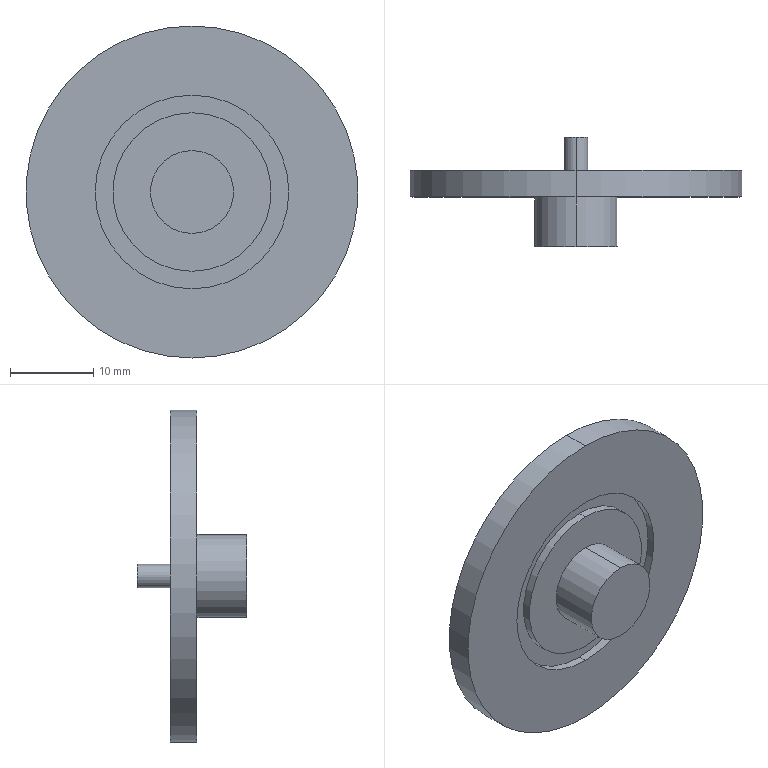Part | SolidWorks | features ICE 5, Extrusion 1 | 1 solid | 28 faces | box 40 x 13.2 x 40 mm | volume 4095 mm3 | cylinder 18 | plane 10 | commonest cylinder face diameters 2.85 x2 10 x2 16.818 x2 19.091 x2 20.068 x2 23.339 x2
STEP:
#1=CARTESIAN_POINT('',(0.,7.2,1.425));
#2=VERTEX_POINT('',#1);
#3=CARTESIAN_POINT('',(0.,7.2,-1.425));
#4=VERTEX_POINT('',#3);
#5=CARTESIAN_POINT('',(0.,7.2,0.));
#6=DIRECTION('',(0.,1.,0.));
#7=DIRECTION('',(0.,0.,1.));
#8=AXIS2_PLACEMENT_3D('',#5,#6,#7);
#9=CIRCLE('',#8,1.425);
#10=EDGE_CURVE('',#2,#4,#9,.T.);
#11=ORIENTED_EDGE('',*,*,#10,.F.);
#12=CARTESIAN_POINT('',(0.,3.2,1.425));
#13=VERTEX_POINT('',#12);
#14=CARTESIAN_POINT('',(0.,7.2,1.425));
#15=DIRECTION('',(0.,-1.,0.));
#16=VECTOR('',#15,1000.);
#17=LINE('',#14,#16);
#18=EDGE_CURVE('',#2,#13,#17,.T.);
#19=ORIENTED_EDGE('',*,*,#18,.T.);
#20=CARTESIAN_POINT('',(0.,3.2,-1.425));
#21=VERTEX_POINT('',#20);
#22=CARTESIAN_POINT('',(0.,3.2,0.));
#23=DIRECTION('',(0.,1.,0.));
#24=DIRECTION('',(0.,0.,1.));
#25=AXIS2_PLACEMENT_3D('',#22,#23,#24);
#26=CIRCLE('',#25,1.425);
#27=EDGE_CURVE('',#13,#21,#26,.T.);
#28=ORIENTED_EDGE('',*,*,#27,.T.);
#29=CARTESIAN_POINT('',(0.,7.2,-1.425));
#30=DIRECTION('',(0.,-1.,0.));
#31=VECTOR('',#30,1000.);
#32=LINE('',#29,#31);
#33=EDGE_CURVE('',#4,#21,#32,.T.);
#34=ORIENTED_EDGE('',*,*,#33,.F.);
#35=EDGE_LOOP('',(#11,#19,#28,#34));
#36=FACE_OUTER_BOUND('',#35,.T.);
#37=CARTESIAN_POINT('',(0.,7.2,0.));
#38=DIRECTION('',(0.,-1.,0.));
#39=DIRECTION('',(0.,0.,-1.));
#40=AXIS2_PLACEMENT_3D('',#37,#38,#39);
#41=CYLINDRICAL_SURFACE('',#40,1.425);
#42=ADVANCED_FACE('',(#36),#41,.T.);
#43=CARTESIAN_POINT('',(0.,2.2,8.409));
#44=VERTEX_POINT('',#43);
#45=CARTESIAN_POINT('',(0.,2.2,-8.409));
#46=VERTEX_POINT('',#45);
#47=CARTESIAN_POINT('',(0.,2.2,0.));
#48=DIRECTION('',(0.,1.,0.));
#49=DIRECTION('',(0.,0.,1.));
#50=AXIS2_PLACEMENT_3D('',#47,#48,#49);
#51=CIRCLE('',#50,8.409);
#52=EDGE_CURVE('',#44,#46,#51,.T.);
#53=ORIENTED_EDGE('',*,*,#52,.T.);
#54=CARTESIAN_POINT('',(0.,3.2,-8.409));
#55=VERTEX_POINT('',#54);
#56=CARTESIAN_POINT('',(0.,2.2,-8.409));
#57=DIRECTION('',(0.,1.,0.));
#58=VECTOR('',#57,1000.);
#59=LINE('',#56,#58);
#60=EDGE_CURVE('',#46,#55,#59,.T.);
#61=ORIENTED_EDGE('',*,*,#60,.T.);
#62=CARTESIAN_POINT('',(0.,3.2,8.409));
#63=VERTEX_POINT('',#62);
#64=CARTESIAN_POINT('',(0.,3.2,0.));
#65=DIRECTION('',(0.,1.,0.));
#66=DIRECTION('',(0.,0.,1.));
#67=AXIS2_PLACEMENT_3D('',#64,#65,#66);
#68=CIRCLE('',#67,8.409);
#69=EDGE_CURVE('',#63,#55,#68,.T.);
#70=ORIENTED_EDGE('',*,*,#69,.F.);
#71=CARTESIAN_POINT('',(0.,2.2,8.409));
#72=DIRECTION('',(0.,1.,0.));
#73=VECTOR('',#72,1000.);
#74=LINE('',#71,#73);
#75=EDGE_CURVE('',#44,#63,#74,.T.);
#76=ORIENTED_EDGE('',*,*,#75,.F.);
#77=EDGE_LOOP('',(#53,#61,#70,#76));
#78=FACE_OUTER_BOUND('',#77,.T.);
#79=CARTESIAN_POINT('',(0.,2.2,0.));
#80=DIRECTION('',(0.,1.,0.));
#81=DIRECTION('',(0.,0.,1.));
#82=AXIS2_PLACEMENT_3D('',#79,#80,#81);
#83=CYLINDRICAL_SURFACE('',#82,8.409);
#84=ADVANCED_FACE('',(#78),#83,.T.);
#85=CARTESIAN_POINT('',(0.,2.2,-10.034));
#86=VERTEX_POINT('',#85);
#87=CARTESIAN_POINT('',(0.,2.2,10.034));
#88=VERTEX_POINT('',#87);
#89=CARTESIAN_POINT('',(0.,2.2,0.));
#90=DIRECTION('',(0.,1.,0.));
#91=DIRECTION('',(0.,0.,1.));
#92=AXIS2_PLACEMENT_3D('',#89,#90,#91);
#93=CIRCLE('',#92,10.034);
#94=EDGE_CURVE('',#86,#88,#93,.T.);
#95=ORIENTED_EDGE('',*,*,#94,.F.);
#96=CARTESIAN_POINT('',(0.,3.2,-10.034));
#97=VERTEX_POINT('',#96);
#98=CARTESIAN_POINT('',(0.,2.2,-10.034));
#99=DIRECTION('',(0.,1.,0.));
#100=VECTOR('',#99,1000.);
#101=LINE('',#98,#100);
#102=EDGE_CURVE('',#86,#97,#101,.T.);
#103=ORIENTED_EDGE('',*,*,#102,.T.);
#104=CARTESIAN_POINT('',(0.,3.2,10.034));
#105=VERTEX_POINT('',#104);
#106=CARTESIAN_POINT('',(0.,3.2,0.));
#107=DIRECTION('',(0.,1.,0.));
#108=DIRECTION('',(0.,0.,1.));
#109=AXIS2_PLACEMENT_3D('',#106,#107,#108);
#110=CIRCLE('',#109,10.034);
#111=EDGE_CURVE('',#97,#105,#110,.T.);
#112=ORIENTED_EDGE('',*,*,#111,.T.);
#113=CARTESIAN_POINT('',(0.,2.2,10.034));
#114=DIRECTION('',(0.,1.,0.));
#115=VECTOR('',#114,1000.);
#116=LINE('',#113,#115);
#117=EDGE_CURVE('',#88,#105,#116,.T.);
#118=ORIENTED_EDGE('',*,*,#117,.F.);
#119=EDGE_LOOP('',(#95,#103,#112,#118));
#120=FACE_OUTER_BOUND('',#119,.T.);
#121=CARTESIAN_POINT('',(0.,2.2,0.));
#122=DIRECTION('',(0.,1.,0.));
#123=DIRECTION('',(0.,0.,1.));
#124=AXIS2_PLACEMENT_3D('',#121,#122,#123);
#125=CYLINDRICAL_SURFACE('',#124,10.034);
#126=ADVANCED_FACE('',(#120),#125,.F.);
#127=CARTESIAN_POINT('',(0.,2.2,15.634));
#128=VERTEX_POINT('',#127);
#129=CARTESIAN_POINT('',(0.,2.2,-15.634));
#130=VERTEX_POINT('',#129);
#131=CARTESIAN_POINT('',(0.,2.2,0.));
#132=DIRECTION('',(0.,1.,0.));
#133=DIRECTION('',(0.,0.,1.));
#134=AXIS2_PLACEMENT_3D('',#131,#132,#133);
#135=CIRCLE('',#134,15.634);
#136=EDGE_CURVE('',#128,#130,#135,.T.);
#137=ORIENTED_EDGE('',*,*,#136,.T.);
#138=CARTESIAN_POINT('',(0.,3.2,-15.634));
#139=VERTEX_POINT('',#138);
#140=CARTESIAN_POINT('',(0.,2.2,-15.634));
#141=DIRECTION('',(0.,1.,0.));
#142=VECTOR('',#141,1000.);
#143=LINE('',#140,#142);
#144=EDGE_CURVE('',#130,#139,#143,.T.);
#145=ORIENTED_EDGE('',*,*,#144,.T.);
#146=CARTESIAN_POINT('',(0.,3.2,15.634));
#147=VERTEX_POINT('',#146);
#148=CARTESIAN_POINT('',(0.,3.2,0.));
#149=DIRECTION('',(0.,1.,0.));
#150=DIRECTION('',(0.,0.,1.));
#151=AXIS2_PLACEMENT_3D('',#148,#149,#150);
#152=CIRCLE('',#151,15.634);
#153=EDGE_CURVE('',#147,#139,#152,.T.);
#154=ORIENTED_EDGE('',*,*,#153,.F.);
#155=CARTESIAN_POINT('',(0.,2.2,15.634));
#156=DIRECTION('',(0.,1.,0.));
#157=VECTOR('',#156,1000.);
#158=LINE('',#155,#157);
#159=EDGE_CURVE('',#128,#147,#158,.T.);
#160=ORIENTED_EDGE('',*,*,#159,.F.);
#161=EDGE_LOOP('',(#137,#145,#154,#160));
#162=FACE_OUTER_BOUND('',#161,.T.);
#163=CARTESIAN_POINT('',(0.,2.2,0.));
#164=DIRECTION('',(0.,1.,0.));
#165=DIRECTION('',(0.,0.,1.));
#166=AXIS2_PLACEMENT_3D('',#163,#164,#165);
#167=CYLINDRICAL_SURFACE('',#166,15.634);
#168=ADVANCED_FACE('',(#162),#167,.T.);
#169=CARTESIAN_POINT('',(0.,2.2,-17.435));
#170=VERTEX_POINT('',#169);
#171=CARTESIAN_POINT('',(0.,2.2,17.435));
#172=VERTEX_POINT('',#171);
#173=CARTESIAN_POINT('',(0.,2.2,0.));
#174=DIRECTION('',(0.,1.,0.));
#175=DIRECTION('',(0.,0.,1.));
#176=AXIS2_PLACEMENT_3D('',#173,#174,#175);
#177=CIRCLE('',#176,17.435);
#178=EDGE_CURVE('',#170,#172,#177,.T.);
#179=ORIENTED_EDGE('',*,*,#178,.F.);
#180=CARTESIAN_POINT('',(0.,3.2,-17.435));
#181=VERTEX_POINT('',#180);
#182=CARTESIAN_POINT('',(0.,2.2,-17.435));
#183=DIRECTION('',(0.,1.,0.));
#184=VECTOR('',#183,1000.);
#185=LINE('',#182,#184);
#186=EDGE_CURVE('',#170,#181,#185,.T.);
#187=ORIENTED_EDGE('',*,*,#186,.T.);
#188=CARTESIAN_POINT('',(0.,3.2,17.435));
#189=VERTEX_POINT('',#188);
#190=CARTESIAN_POINT('',(0.,3.2,0.));
#191=DIRECTION('',(0.,1.,0.));
#192=DIRECTION('',(0.,0.,1.));
#193=AXIS2_PLACEMENT_3D('',#190,#191,#192);
#194=CIRCLE('',#193,17.435);
#195=EDGE_CURVE('',#181,#189,#194,.T.);
#196=ORIENTED_EDGE('',*,*,#195,.T.);
#197=CARTESIAN_POINT('',(0.,2.2,17.435));
#198=DIRECTION('',(0.,1.,0.));
#199=VECTOR('',#198,1000.);
#200=LINE('',#197,#199);
#201=EDGE_CURVE('',#172,#189,#200,.T.);
#202=ORIENTED_EDGE('',*,*,#201,.F.);
#203=EDGE_LOOP('',(#179,#187,#196,#202));
#204=FACE_OUTER_BOUND('',#203,.T.);
#205=CARTESIAN_POINT('',(0.,2.2,0.));
#206=DIRECTION('',(0.,1.,0.));
#207=DIRECTION('',(0.,0.,1.));
#208=AXIS2_PLACEMENT_3D('',#205,#206,#207);
#209=CYLINDRICAL_SURFACE('',#208,17.435);
#210=ADVANCED_FACE('',(#204),#209,.F.);
#211=CARTESIAN_POINT('',(0.,-6.,-5.));
#212=VERTEX_POINT('',#211);
#213=CARTESIAN_POINT('',(0.,-6.,5.));
#214=VERTEX_POINT('',#213);
#215=CARTESIAN_POINT('',(0.,-6.,0.));
#216=DIRECTION('',(0.,-1.,0.));
#217=DIRECTION('',(0.,0.,-1.));
#218=AXIS2_PLACEMENT_3D('',#215,#216,#217);
#219=CIRCLE('',#218,5.);
#220=EDGE_CURVE('',#212,#214,#219,.T.);
#221=ORIENTED_EDGE('',*,*,#220,.F.);
#222=CARTESIAN_POINT('',(0.,0.,-5.));
#223=VERTEX_POINT('',#222);
#224=CARTESIAN_POINT('',(0.,-6.,-5.));
#225=DIRECTION('',(0.,1.,0.));
#226=VECTOR('',#225,1000.);
#227=LINE('',#224,#226);
#228=EDGE_CURVE('',#212,#223,#227,.T.);
#229=ORIENTED_EDGE('',*,*,#228,.T.);
#230=CARTESIAN_POINT('',(0.,0.,5.));
#231=VERTEX_POINT('',#230);
#232=CARTESIAN_POINT('',(0.,0.,0.));
#233=DIRECTION('',(0.,-1.,0.));
#234=DIRECTION('',(0.,0.,-1.));
#235=AXIS2_PLACEMENT_3D('',#232,#233,#234);
#236=CIRCLE('',#235,5.);
#237=EDGE_CURVE('',#223,#231,#236,.T.);
#238=ORIENTED_EDGE('',*,*,#237,.T.);
#239=CARTESIAN_POINT('',(0.,-6.,5.));
#240=DIRECTION('',(0.,1.,0.));
#241=VECTOR('',#240,1000.);
#242=LINE('',#239,#241);
#243=EDGE_CURVE('',#214,#231,#242,.T.);
#244=ORIENTED_EDGE('',*,*,#243,.F.);
#245=EDGE_LOOP('',(#221,#229,#238,#244));
#246=FACE_OUTER_BOUND('',#245,.T.);
#247=CARTESIAN_POINT('',(0.,-6.,0.));
#248=DIRECTION('',(0.,1.,0.));
#249=DIRECTION('',(0.,0.,1.));
#250=AXIS2_PLACEMENT_3D('',#247,#248,#249);
#251=CYLINDRICAL_SURFACE('',#250,5.);
#252=ADVANCED_FACE('',(#246),#251,.T.);
#253=CARTESIAN_POINT('',(0.,1.,-9.545));
#254=VERTEX_POINT('',#253);
#255=CARTESIAN_POINT('',(0.,1.,9.545));
#256=VERTEX_POINT('',#255);
#257=CARTESIAN_POINT('',(0.,1.,0.));
#258=DIRECTION('',(0.,-1.,0.));
#259=DIRECTION('',(0.,0.,-1.));
#260=AXIS2_PLACEMENT_3D('',#257,#258,#259);
#261=CIRCLE('',#260,9.545);
#262=EDGE_CURVE('',#254,#256,#261,.T.);
#263=ORIENTED_EDGE('',*,*,#262,.T.);
#264=CARTESIAN_POINT('',(0.,0.,9.545));
#265=VERTEX_POINT('',#264);
#266=CARTESIAN_POINT('',(0.,1.,9.545));
#267=DIRECTION('',(0.,-1.,0.));
#268=VECTOR('',#267,1000.);
#269=LINE('',#266,#268);
#270=EDGE_CURVE('',#256,#265,#269,.T.);
#271=ORIENTED_EDGE('',*,*,#270,.T.);
#272=CARTESIAN_POINT('',(0.,0.,-9.545));
#273=VERTEX_POINT('',#272);
#274=CARTESIAN_POINT('',(0.,0.,0.));
#275=DIRECTION('',(0.,-1.,0.));
#276=DIRECTION('',(0.,0.,-1.));
#277=AXIS2_PLACEMENT_3D('',#274,#275,#276);
#278=CIRCLE('',#277,9.545);
#279=EDGE_CURVE('',#273,#265,#278,.T.);
#280=ORIENTED_EDGE('',*,*,#279,.F.);
#281=CARTESIAN_POINT('',(0.,1.,-9.545));
#282=DIRECTION('',(0.,-1.,0.));
#283=VECTOR('',#282,1000.);
#284=LINE('',#281,#283);
#285=EDGE_CURVE('',#254,#273,#284,.T.);
#286=ORIENTED_EDGE('',*,*,#285,.F.);
#287=EDGE_LOOP('',(#263,#271,#280,#286));
#288=FACE_OUTER_BOUND('',#287,.T.);
#289=CARTESIAN_POINT('',(0.,1.,0.));
#290=DIRECTION('',(0.,-1.,0.));
#291=DIRECTION('',(0.,0.,-1.));
#292=AXIS2_PLACEMENT_3D('',#289,#290,#291);
#293=CYLINDRICAL_SURFACE('',#292,9.545);
#294=ADVANCED_FACE('',(#288),#293,.T.);
#295=CARTESIAN_POINT('',(0.,1.,11.669));
#296=VERTEX_POINT('',#295);
#297=CARTESIAN_POINT('',(0.,1.,-11.669));
#298=VERTEX_POINT('',#297);
#299=CARTESIAN_POINT('',(0.,1.,0.));
#300=DIRECTION('',(0.,-1.,0.));
#301=DIRECTION('',(0.,0.,-1.));
#302=AXIS2_PLACEMENT_3D('',#299,#300,#301);
#303=CIRCLE('',#302,11.669);
#304=EDGE_CURVE('',#296,#298,#303,.T.);
#305=ORIENTED_EDGE('',*,*,#304,.F.);
#306=CARTESIAN_POINT('',(0.,0.,11.669));
#307=VERTEX_POINT('',#306);
#308=CARTESIAN_POINT('',(0.,1.,11.669));
#309=DIRECTION('',(0.,-1.,0.));
#310=VECTOR('',#309,1000.);
#311=LINE('',#308,#310);
#312=EDGE_CURVE('',#296,#307,#311,.T.);
#313=ORIENTED_EDGE('',*,*,#312,.T.);
#314=CARTESIAN_POINT('',(0.,0.,-11.669));
#315=VERTEX_POINT('',#314);
#316=CARTESIAN_POINT('',(0.,0.,0.));
#317=DIRECTION('',(0.,-1.,0.));
#318=DIRECTION('',(0.,0.,-1.));
#319=AXIS2_PLACEMENT_3D('',#316,#317,#318);
#320=CIRCLE('',#319,11.669);
#321=EDGE_CURVE('',#307,#315,#320,.T.);
#322=ORIENTED_EDGE('',*,*,#321,.T.);
#323=CARTESIAN_POINT('',(0.,1.,-11.669));
#324=DIRECTION('',(0.,-1.,0.));
#325=VECTOR('',#324,1000.);
#326=LINE('',#323,#325);
#327=EDGE_CURVE('',#298,#315,#326,.T.);
#328=ORIENTED_EDGE('',*,*,#327,.F.);
#329=EDGE_LOOP('',(#305,#313,#322,#328));
#330=FACE_OUTER_BOUND('',#329,.T.);
#331=CARTESIAN_POINT('',(0.,1.,0.));
#332=DIRECTION('',(0.,-1.,0.));
#333=DIRECTION('',(0.,0.,-1.));
#334=AXIS2_PLACEMENT_3D('',#331,#332,#333);
#335=CYLINDRICAL_SURFACE('',#334,11.669);
#336=ADVANCED_FACE('',(#330),#335,.F.);
#337=CARTESIAN_POINT('',(0.,3.2,20.));
#338=VERTEX_POINT('',#337);
#339=CARTESIAN_POINT('',(0.,3.2,-20.));
#340=VERTEX_POINT('',#339);
#341=CARTESIAN_POINT('',(0.,3.2,0.));
#342=DIRECTION('',(0.,1.,0.));
#343=DIRECTION('',(0.,0.,1.));
#344=AXIS2_PLACEMENT_3D('',#341,#342,#343);
#345=CIRCLE('',#344,20.);
#346=EDGE_CURVE('',#338,#340,#345,.T.);
#347=ORIENTED_EDGE('',*,*,#346,.F.);
#348=CARTESIAN_POINT('',(0.,0.,20.));
#349=VERTEX_POINT('',#348);
#350=CARTESIAN_POINT('',(0.,3.2,20.));
#351=DIRECTION('',(0.,-1.,0.));
#352=VECTOR('',#351,1000.);
#353=LINE('',#350,#352);
#354=EDGE_CURVE('',#338,#349,#353,.T.);
#355=ORIENTED_EDGE('',*,*,#354,.T.);
#356=CARTESIAN_POINT('',(0.,0.,-20.));
#357=VERTEX_POINT('',#356);
#358=CARTESIAN_POINT('',(0.,0.,0.));
#359=DIRECTION('',(0.,1.,0.));
#360=DIRECTION('',(0.,0.,1.));
#361=AXIS2_PLACEMENT_3D('',#358,#359,#360);
#362=CIRCLE('',#361,20.);
#363=EDGE_CURVE('',#349,#357,#362,.T.);
#364=ORIENTED_EDGE('',*,*,#363,.T.);
#365=CARTESIAN_POINT('',(0.,3.2,-20.));
#366=DIRECTION('',(0.,-1.,0.));
#367=VECTOR('',#366,1000.);
#368=LINE('',#365,#367);
#369=EDGE_CURVE('',#340,#357,#368,.T.);
#370=ORIENTED_EDGE('',*,*,#369,.F.);
#371=EDGE_LOOP('',(#347,#355,#364,#370));
#372=FACE_OUTER_BOUND('',#371,.T.);
#373=CARTESIAN_POINT('',(0.,3.2,0.));
#374=DIRECTION('',(0.,-1.,0.));
#375=DIRECTION('',(0.,0.,-1.));
#376=AXIS2_PLACEMENT_3D('',#373,#374,#375);
#377=CYLINDRICAL_SURFACE('',#376,20.);
#378=ADVANCED_FACE('',(#372),#377,.T.);
#379=ORIENTED_EDGE('',*,*,#354,.F.);
#380=CARTESIAN_POINT('',(0.,3.2,0.));
#381=DIRECTION('',(0.,1.,0.));
#382=DIRECTION('',(0.,0.,1.));
#383=AXIS2_PLACEMENT_3D('',#380,#381,#382);
#384=CIRCLE('',#383,20.);
#385=EDGE_CURVE('',#340,#338,#384,.T.);
#386=ORIENTED_EDGE('',*,*,#385,.F.);
#387=ORIENTED_EDGE('',*,*,#369,.T.);
#388=CARTESIAN_POINT('',(0.,0.,0.));
#389=DIRECTION('',(0.,1.,0.));
#390=DIRECTION('',(0.,0.,1.));
#391=AXIS2_PLACEMENT_3D('',#388,#389,#390);
#392=CIRCLE('',#391,20.);
#393=EDGE_CURVE('',#357,#349,#392,.T.);
#394=ORIENTED_EDGE('',*,*,#393,.T.);
#395=EDGE_LOOP('',(#379,#386,#387,#394));
#396=FACE_OUTER_BOUND('',#395,.T.);
#397=CARTESIAN_POINT('',(0.,3.2,0.));
#398=DIRECTION('',(0.,-1.,0.));
#399=DIRECTION('',(0.,0.,-1.));
#400=AXIS2_PLACEMENT_3D('',#397,#398,#399);
#401=CYLINDRICAL_SURFACE('',#400,20.);
#402=ADVANCED_FACE('',(#396),#401,.T.);
#403=CARTESIAN_POINT('',(0.,3.2,0.));
#404=DIRECTION('',(0.,1.,0.));
#405=DIRECTION('',(0.,0.,1.));
#406=AXIS2_PLACEMENT_3D('',#403,#404,#405);
#407=CIRCLE('',#406,17.435);
#408=EDGE_CURVE('',#189,#181,#407,.T.);
#409=ORIENTED_EDGE('',*,*,#408,.F.);
#410=ORIENTED_EDGE('',*,*,#195,.F.);
#411=EDGE_LOOP('',(#409,#410));
#412=FACE_BOUND('',#411,.T.);
#413=ORIENTED_EDGE('',*,*,#385,.T.);
#414=ORIENTED_EDGE('',*,*,#346,.T.);
#415=EDGE_LOOP('',(#413,#414));
#416=FACE_OUTER_BOUND('',#415,.T.);
#417=CARTESIAN_POINT('',(0.,3.2,0.));
#418=DIRECTION('',(0.,1.,0.));
#419=DIRECTION('',(0.,0.,1.));
#420=AXIS2_PLACEMENT_3D('',#417,#418,#419);
#421=PLANE('',#420);
#422=ADVANCED_FACE('',(#412,#416),#421,.T.);
#423=CARTESIAN_POINT('',(0.,0.,0.));
#424=DIRECTION('',(0.,-1.,0.));
#425=DIRECTION('',(0.,0.,-1.));
#426=AXIS2_PLACEMENT_3D('',#423,#424,#425);
#427=CIRCLE('',#426,11.669);
#428=EDGE_CURVE('',#315,#307,#427,.T.);
#429=ORIENTED_EDGE('',*,*,#428,.F.);
#430=ORIENTED_EDGE('',*,*,#321,.F.);
#431=EDGE_LOOP('',(#429,#430));
#432=FACE_BOUND('',#431,.T.);
#433=ORIENTED_EDGE('',*,*,#393,.F.);
#434=ORIENTED_EDGE('',*,*,#363,.F.);
#435=EDGE_LOOP('',(#433,#434));
#436=FACE_OUTER_BOUND('',#435,.T.);
#437=CARTESIAN_POINT('',(0.,0.,0.));
#438=DIRECTION('',(0.,1.,0.));
#439=DIRECTION('',(0.,0.,1.));
#440=AXIS2_PLACEMENT_3D('',#437,#438,#439);
#441=PLANE('',#440);
#442=ADVANCED_FACE('',(#432,#436),#441,.F.);
#443=ORIENTED_EDGE('',*,*,#312,.F.);
#444=CARTESIAN_POINT('',(0.,1.,0.));
#445=DIRECTION('',(0.,-1.,0.));
#446=DIRECTION('',(0.,0.,-1.));
#447=AXIS2_PLACEMENT_3D('',#444,#445,#446);
#448=CIRCLE('',#447,11.669);
#449=EDGE_CURVE('',#298,#296,#448,.T.);
#450=ORIENTED_EDGE('',*,*,#449,.F.);
#451=ORIENTED_EDGE('',*,*,#327,.T.);
#452=ORIENTED_EDGE('',*,*,#428,.T.);
#453=EDGE_LOOP('',(#443,#450,#451,#452));
#454=FACE_OUTER_BOUND('',#453,.T.);
#455=CARTESIAN_POINT('',(0.,1.,0.));
#456=DIRECTION('',(0.,-1.,0.));
#457=DIRECTION('',(0.,0.,-1.));
#458=AXIS2_PLACEMENT_3D('',#455,#456,#457);
#459=CYLINDRICAL_SURFACE('',#458,11.669);
#460=ADVANCED_FACE('',(#454),#459,.F.);
#461=ORIENTED_EDGE('',*,*,#262,.F.);
#462=CARTESIAN_POINT('',(0.,1.,0.));
#463=DIRECTION('',(0.,-1.,0.));
#464=DIRECTION('',(0.,0.,-1.));
#465=AXIS2_PLACEMENT_3D('',#462,#463,#464);
#466=CIRCLE('',#465,9.545);
#467=EDGE_CURVE('',#256,#254,#466,.T.);
#468=ORIENTED_EDGE('',*,*,#467,.F.);
#469=EDGE_LOOP('',(#461,#468));
#470=FACE_BOUND('',#469,.T.);
#471=ORIENTED_EDGE('',*,*,#449,.T.);
#472=ORIENTED_EDGE('',*,*,#304,.T.);
#473=EDGE_LOOP('',(#471,#472));
#474=FACE_OUTER_BOUND('',#473,.T.);
#475=CARTESIAN_POINT('',(0.,1.,0.));
#476=DIRECTION('',(0.,-1.,0.));
#477=DIRECTION('',(0.,0.,-1.));
#478=AXIS2_PLACEMENT_3D('',#475,#476,#477);
#479=PLANE('',#478);
#480=ADVANCED_FACE('',(#470,#474),#479,.T.);
#481=ORIENTED_EDGE('',*,*,#270,.F.);
#482=ORIENTED_EDGE('',*,*,#467,.T.);
#483=ORIENTED_EDGE('',*,*,#285,.T.);
#484=CARTESIAN_POINT('',(0.,0.,0.));
#485=DIRECTION('',(0.,-1.,0.));
#486=DIRECTION('',(0.,0.,-1.));
#487=AXIS2_PLACEMENT_3D('',#484,#485,#486);
#488=CIRCLE('',#487,9.545);
#489=EDGE_CURVE('',#265,#273,#488,.T.);
#490=ORIENTED_EDGE('',*,*,#489,.F.);
#491=EDGE_LOOP('',(#481,#482,#483,#490));
#492=FACE_OUTER_BOUND('',#491,.T.);
#493=CARTESIAN_POINT('',(0.,1.,0.));
#494=DIRECTION('',(0.,-1.,0.));
#495=DIRECTION('',(0.,0.,-1.));
#496=AXIS2_PLACEMENT_3D('',#493,#494,#495);
#497=CYLINDRICAL_SURFACE('',#496,9.545);
#498=ADVANCED_FACE('',(#492),#497,.T.);
#499=CARTESIAN_POINT('',(0.,-6.,0.));
#500=DIRECTION('',(0.,-1.,0.));
#501=DIRECTION('',(0.,0.,-1.));
#502=AXIS2_PLACEMENT_3D('',#499,#500,#501);
#503=CIRCLE('',#502,5.);
#504=EDGE_CURVE('',#214,#212,#503,.T.);
#505=ORIENTED_EDGE('',*,*,#504,.T.);
#506=ORIENTED_EDGE('',*,*,#220,.T.);
#507=EDGE_LOOP('',(#505,#506));
#508=FACE_OUTER_BOUND('',#507,.T.);
#509=CARTESIAN_POINT('',(0.,-6.,0.));
#510=DIRECTION('',(0.,-1.,0.));
#511=DIRECTION('',(0.,0.,-1.));
#512=AXIS2_PLACEMENT_3D('',#509,#510,#511);
#513=PLANE('',#512);
#514=ADVANCED_FACE('',(#508),#513,.T.);
#515=ORIENTED_EDGE('',*,*,#228,.F.);
#516=ORIENTED_EDGE('',*,*,#504,.F.);
#517=ORIENTED_EDGE('',*,*,#243,.T.);
#518=CARTESIAN_POINT('',(0.,0.,0.));
#519=DIRECTION('',(0.,-1.,0.));
#520=DIRECTION('',(0.,0.,-1.));
#521=AXIS2_PLACEMENT_3D('',#518,#519,#520);
#522=CIRCLE('',#521,5.);
#523=EDGE_CURVE('',#231,#223,#522,.T.);
#524=ORIENTED_EDGE('',*,*,#523,.T.);
#525=EDGE_LOOP('',(#515,#516,#517,#524));
#526=FACE_OUTER_BOUND('',#525,.T.);
#527=CARTESIAN_POINT('',(0.,-6.,0.));
#528=DIRECTION('',(0.,1.,0.));
#529=DIRECTION('',(0.,0.,1.));
#530=AXIS2_PLACEMENT_3D('',#527,#528,#529);
#531=CYLINDRICAL_SURFACE('',#530,5.);
#532=ADVANCED_FACE('',(#526),#531,.T.);
#533=ORIENTED_EDGE('',*,*,#523,.F.);
#534=ORIENTED_EDGE('',*,*,#237,.F.);
#535=EDGE_LOOP('',(#533,#534));
#536=FACE_BOUND('',#535,.T.);
#537=ORIENTED_EDGE('',*,*,#279,.T.);
#538=ORIENTED_EDGE('',*,*,#489,.T.);
#539=EDGE_LOOP('',(#537,#538));
#540=FACE_OUTER_BOUND('',#539,.T.);
#541=CARTESIAN_POINT('',(0.,0.,0.));
#542=DIRECTION('',(0.,1.,0.));
#543=DIRECTION('',(0.,0.,1.));
#544=AXIS2_PLACEMENT_3D('',#541,#542,#543);
#545=PLANE('',#544);
#546=ADVANCED_FACE('',(#536,#540),#545,.F.);
#547=ORIENTED_EDGE('',*,*,#186,.F.);
#548=CARTESIAN_POINT('',(0.,2.2,0.));
#549=DIRECTION('',(0.,1.,0.));
#550=DIRECTION('',(0.,0.,1.));
#551=AXIS2_PLACEMENT_3D('',#548,#549,#550);
#552=CIRCLE('',#551,17.435);
#553=EDGE_CURVE('',#172,#170,#552,.T.);
#554=ORIENTED_EDGE('',*,*,#553,.F.);
#555=ORIENTED_EDGE('',*,*,#201,.T.);
#556=ORIENTED_EDGE('',*,*,#408,.T.);
#557=EDGE_LOOP('',(#547,#554,#555,#556));
#558=FACE_OUTER_BOUND('',#557,.T.);
#559=CARTESIAN_POINT('',(0.,2.2,0.));
#560=DIRECTION('',(0.,1.,0.));
#561=DIRECTION('',(0.,0.,1.));
#562=AXIS2_PLACEMENT_3D('',#559,#560,#561);
#563=CYLINDRICAL_SURFACE('',#562,17.435);
#564=ADVANCED_FACE('',(#558),#563,.F.);
#565=ORIENTED_EDGE('',*,*,#136,.F.);
#566=CARTESIAN_POINT('',(0.,2.2,0.));
#567=DIRECTION('',(0.,1.,0.));
#568=DIRECTION('',(0.,0.,1.));
#569=AXIS2_PLACEMENT_3D('',#566,#567,#568);
#570=CIRCLE('',#569,15.634);
#571=EDGE_CURVE('',#130,#128,#570,.T.);
#572=ORIENTED_EDGE('',*,*,#571,.F.);
#573=EDGE_LOOP('',(#565,#572));
#574=FACE_BOUND('',#573,.T.);
#575=ORIENTED_EDGE('',*,*,#553,.T.);
#576=ORIENTED_EDGE('',*,*,#178,.T.);
#577=EDGE_LOOP('',(#575,#576));
#578=FACE_OUTER_BOUND('',#577,.T.);
#579=CARTESIAN_POINT('',(0.,2.2,0.));
#580=DIRECTION('',(0.,1.,0.));
#581=DIRECTION('',(0.,0.,1.));
#582=AXIS2_PLACEMENT_3D('',#579,#580,#581);
#583=PLANE('',#582);
#584=ADVANCED_FACE('',(#574,#578),#583,.T.);
#585=ORIENTED_EDGE('',*,*,#144,.F.);
#586=ORIENTED_EDGE('',*,*,#571,.T.);
#587=ORIENTED_EDGE('',*,*,#159,.T.);
#588=CARTESIAN_POINT('',(0.,3.2,0.));
#589=DIRECTION('',(0.,1.,0.));
#590=DIRECTION('',(0.,0.,1.));
#591=AXIS2_PLACEMENT_3D('',#588,#589,#590);
#592=CIRCLE('',#591,15.634);
#593=EDGE_CURVE('',#139,#147,#592,.T.);
#594=ORIENTED_EDGE('',*,*,#593,.F.);
#595=EDGE_LOOP('',(#585,#586,#587,#594));
#596=FACE_OUTER_BOUND('',#595,.T.);
#597=CARTESIAN_POINT('',(0.,2.2,0.));
#598=DIRECTION('',(0.,1.,0.));
#599=DIRECTION('',(0.,0.,1.));
#600=AXIS2_PLACEMENT_3D('',#597,#598,#599);
#601=CYLINDRICAL_SURFACE('',#600,15.634);
#602=ADVANCED_FACE('',(#596),#601,.T.);
#603=CARTESIAN_POINT('',(0.,3.2,0.));
#604=DIRECTION('',(0.,1.,0.));
#605=DIRECTION('',(0.,0.,1.));
#606=AXIS2_PLACEMENT_3D('',#603,#604,#605);
#607=CIRCLE('',#606,10.034);
#608=EDGE_CURVE('',#105,#97,#607,.T.);
#609=ORIENTED_EDGE('',*,*,#608,.F.);
#610=ORIENTED_EDGE('',*,*,#111,.F.);
#611=EDGE_LOOP('',(#609,#610));
#612=FACE_BOUND('',#611,.T.);
#613=ORIENTED_EDGE('',*,*,#153,.T.);
#614=ORIENTED_EDGE('',*,*,#593,.T.);
#615=EDGE_LOOP('',(#613,#614));
#616=FACE_OUTER_BOUND('',#615,.T.);
#617=CARTESIAN_POINT('',(0.,3.2,0.));
#618=DIRECTION('',(0.,1.,0.));
#619=DIRECTION('',(0.,0.,1.));
#620=AXIS2_PLACEMENT_3D('',#617,#618,#619);
#621=PLANE('',#620);
#622=ADVANCED_FACE('',(#612,#616),#621,.T.);
#623=ORIENTED_EDGE('',*,*,#102,.F.);
#624=CARTESIAN_POINT('',(0.,2.2,0.));
#625=DIRECTION('',(0.,1.,0.));
#626=DIRECTION('',(0.,0.,1.));
#627=AXIS2_PLACEMENT_3D('',#624,#625,#626);
#628=CIRCLE('',#627,10.034);
#629=EDGE_CURVE('',#88,#86,#628,.T.);
#630=ORIENTED_EDGE('',*,*,#629,.F.);
#631=ORIENTED_EDGE('',*,*,#117,.T.);
#632=ORIENTED_EDGE('',*,*,#608,.T.);
#633=EDGE_LOOP('',(#623,#630,#631,#632));
#634=FACE_OUTER_BOUND('',#633,.T.);
#635=CARTESIAN_POINT('',(0.,2.2,0.));
#636=DIRECTION('',(0.,1.,0.));
#637=DIRECTION('',(0.,0.,1.));
#638=AXIS2_PLACEMENT_3D('',#635,#636,#637);
#639=CYLINDRICAL_SURFACE('',#638,10.034);
#640=ADVANCED_FACE('',(#634),#639,.F.);
#641=ORIENTED_EDGE('',*,*,#52,.F.);
#642=CARTESIAN_POINT('',(0.,2.2,0.));
#643=DIRECTION('',(0.,1.,0.));
#644=DIRECTION('',(0.,0.,1.));
#645=AXIS2_PLACEMENT_3D('',#642,#643,#644);
#646=CIRCLE('',#645,8.409);
#647=EDGE_CURVE('',#46,#44,#646,.T.);
#648=ORIENTED_EDGE('',*,*,#647,.F.);
#649=EDGE_LOOP('',(#641,#648));
#650=FACE_BOUND('',#649,.T.);
#651=ORIENTED_EDGE('',*,*,#629,.T.);
#652=ORIENTED_EDGE('',*,*,#94,.T.);
#653=EDGE_LOOP('',(#651,#652));
#654=FACE_OUTER_BOUND('',#653,.T.);
#655=CARTESIAN_POINT('',(0.,2.2,0.));
#656=DIRECTION('',(0.,1.,0.));
#657=DIRECTION('',(0.,0.,1.));
#658=AXIS2_PLACEMENT_3D('',#655,#656,#657);
#659=PLANE('',#658);
#660=ADVANCED_FACE('',(#650,#654),#659,.T.);
#661=ORIENTED_EDGE('',*,*,#60,.F.);
#662=ORIENTED_EDGE('',*,*,#647,.T.);
#663=ORIENTED_EDGE('',*,*,#75,.T.);
#664=CARTESIAN_POINT('',(0.,3.2,0.));
#665=DIRECTION('',(0.,1.,0.));
#666=DIRECTION('',(0.,0.,1.));
#667=AXIS2_PLACEMENT_3D('',#664,#665,#666);
#668=CIRCLE('',#667,8.409);
#669=EDGE_CURVE('',#55,#63,#668,.T.);
#670=ORIENTED_EDGE('',*,*,#669,.F.);
#671=EDGE_LOOP('',(#661,#662,#663,#670));
#672=FACE_OUTER_BOUND('',#671,.T.);
#673=CARTESIAN_POINT('',(0.,2.2,0.));
#674=DIRECTION('',(0.,1.,0.));
#675=DIRECTION('',(0.,0.,1.));
#676=AXIS2_PLACEMENT_3D('',#673,#674,#675);
#677=CYLINDRICAL_SURFACE('',#676,8.409);
#678=ADVANCED_FACE('',(#672),#677,.T.);
#679=CARTESIAN_POINT('',(0.,7.2,0.));
#680=DIRECTION('',(0.,1.,0.));
#681=DIRECTION('',(0.,0.,1.));
#682=AXIS2_PLACEMENT_3D('',#679,#680,#681);
#683=CIRCLE('',#682,1.425);
#684=EDGE_CURVE('',#4,#2,#683,.T.);
#685=ORIENTED_EDGE('',*,*,#684,.T.);
#686=ORIENTED_EDGE('',*,*,#10,.T.);
#687=EDGE_LOOP('',(#685,#686));
#688=FACE_OUTER_BOUND('',#687,.T.);
#689=CARTESIAN_POINT('',(0.,7.2,0.));
#690=DIRECTION('',(0.,1.,0.));
#691=DIRECTION('',(0.,0.,1.));
#692=AXIS2_PLACEMENT_3D('',#689,#690,#691);
#693=PLANE('',#692);
#694=ADVANCED_FACE('',(#688),#693,.T.);
#695=ORIENTED_EDGE('',*,*,#18,.F.);
#696=ORIENTED_EDGE('',*,*,#684,.F.);
#697=ORIENTED_EDGE('',*,*,#33,.T.);
#698=CARTESIAN_POINT('',(0.,3.2,0.));
#699=DIRECTION('',(0.,1.,0.));
#700=DIRECTION('',(0.,0.,1.));
#701=AXIS2_PLACEMENT_3D('',#698,#699,#700);
#702=CIRCLE('',#701,1.425);
#703=EDGE_CURVE('',#21,#13,#702,.T.);
#704=ORIENTED_EDGE('',*,*,#703,.T.);
#705=EDGE_LOOP('',(#695,#696,#697,#704));
#706=FACE_OUTER_BOUND('',#705,.T.);
#707=CARTESIAN_POINT('',(0.,7.2,0.));
#708=DIRECTION('',(0.,-1.,0.));
#709=DIRECTION('',(0.,0.,-1.));
#710=AXIS2_PLACEMENT_3D('',#707,#708,#709);
#711=CYLINDRICAL_SURFACE('',#710,1.425);
#712=ADVANCED_FACE('',(#706),#711,.T.);
#713=ORIENTED_EDGE('',*,*,#703,.F.);
#714=ORIENTED_EDGE('',*,*,#27,.F.);
#715=EDGE_LOOP('',(#713,#714));
#716=FACE_BOUND('',#715,.T.);
#717=ORIENTED_EDGE('',*,*,#69,.T.);
#718=ORIENTED_EDGE('',*,*,#669,.T.);
#719=EDGE_LOOP('',(#717,#718));
#720=FACE_OUTER_BOUND('',#719,.T.);
#721=CARTESIAN_POINT('',(0.,3.2,0.));
#722=DIRECTION('',(0.,1.,0.));
#723=DIRECTION('',(0.,0.,1.));
#724=AXIS2_PLACEMENT_3D('',#721,#722,#723);
#725=PLANE('',#724);
#726=ADVANCED_FACE('',(#716,#720),#725,.T.);
#727=CLOSED_SHELL('',(#42,#84,#126,#168,#210,#252,#294,#336,#378,#402,#422,#442,#460,#480,#498,#514,#532,#546,#564,#584,#602,#622,#640,#660,#678,#694,#712,#726));
#728=MANIFOLD_SOLID_BREP('',#727);
#729=CARTESIAN_POINT('',(0.,0.,0.));
#730=DIRECTION('',(0.,0.,1.));
#731=DIRECTION('',(1.,0.,0.));
#732=AXIS2_PLACEMENT_3D('',#729,#730,#731);
#733=(LENGTH_UNIT()NAMED_UNIT(*)SI_UNIT(.MILLI.,.METRE.));
#734=UNCERTAINTY_MEASURE_WITH_UNIT(LENGTH_MEASURE(0.00001),#733,'','');
#735=(NAMED_UNIT(*)PLANE_ANGLE_UNIT()SI_UNIT($,.RADIAN.));
#736=(NAMED_UNIT(*)SI_UNIT($,.STERADIAN.)SOLID_ANGLE_UNIT());
#737=(GEOMETRIC_REPRESENTATION_CONTEXT(3)GLOBAL_UNCERTAINTY_ASSIGNED_CONTEXT((#734))GLOBAL_UNIT_ASSIGNED_CONTEXT((#733,#735,#736))REPRESENTATION_CONTEXT('',''));
#738=ADVANCED_BREP_SHAPE_REPRESENTATION('',(#728,#732),#737);